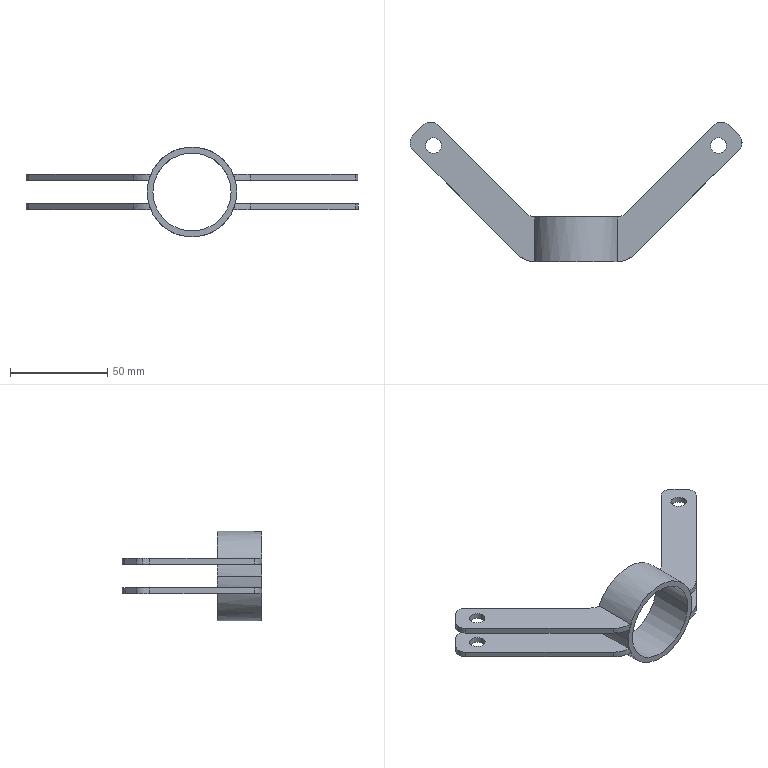Part | SolidWorks | features ICE 3, CosmeticWeldCutList 1, Extrusion 1 | 1 solid | 55 faces | box 170.316 x 71.647 x 46.1 mm | volume 26521 mm3 | cylinder 30 | plane 25 | commonest cylinder face diameters 10 x10 8 x8 14 x4 26 x4 40.1 x2 46.1 x2